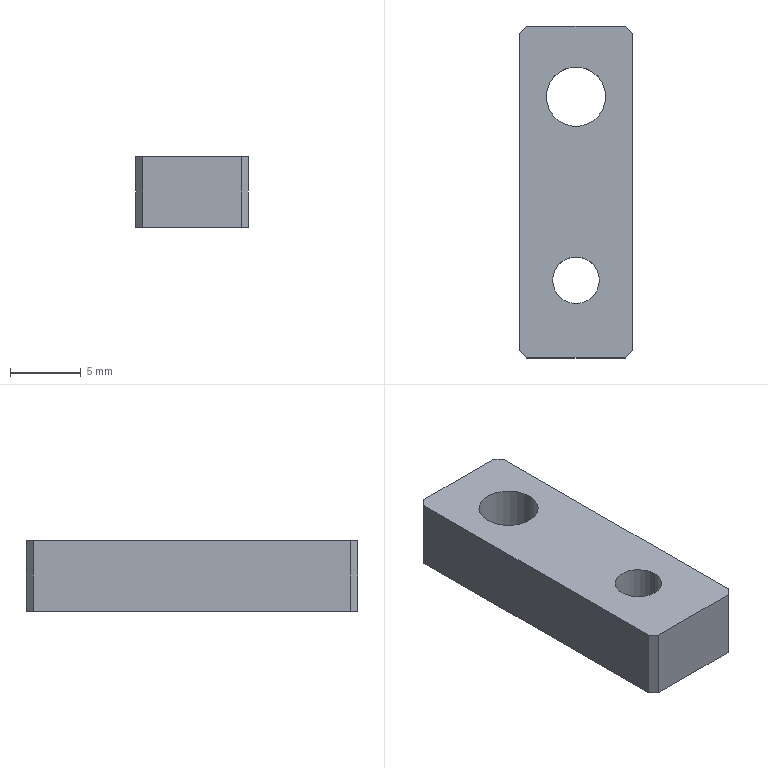Part | STEP file | 1 solid | 14 faces | box 8 x 23.5 x 5 mm | volume 825.463 mm3 | plane 10 | cylinder 4 | commonest cylinder face diameters 3.3 x2 4.2 x2
STEP:
#1=CARTESIAN_POINT('',(0.,0.,0.));
#2=DIRECTION('',(0.,0.,1.));
#3=DIRECTION('',(1.,0.,0.));
#4=AXIS2_PLACEMENT_3D('',#1,#2,#3);
#5=CARTESIAN_POINT('',(2.1,6.75,0.));
#6=VERTEX_POINT('',#5);
#7=CARTESIAN_POINT('',(2.1,6.75,5.));
#8=VERTEX_POINT('',#7);
#9=CARTESIAN_POINT('',(2.1,6.75,5.));
#10=DIRECTION('',(0.,0.,1.));
#11=VECTOR('',#10,1.);
#12=LINE('',#9,#11);
#13=CARTESIAN_POINT('',(0.,6.75,5.));
#14=DIRECTION('',(0.,0.,1.));
#15=DIRECTION('',(1.,0.,0.));
#16=AXIS2_PLACEMENT_3D('',#13,#14,#15);
#17=CYLINDRICAL_SURFACE('',#16,2.1);
#18=CARTESIAN_POINT('',(6.283,0.));
#19=DIRECTION('',(0.,1.));
#20=VECTOR('',#19,1.);
#21=LINE('',#18,#20);
#22=(GEOMETRIC_REPRESENTATION_CONTEXT(2)PARAMETRIC_REPRESENTATION_CONTEXT()REPRESENTATION_CONTEXT('',''));
#23=DEFINITIONAL_REPRESENTATION('',(#21),#22);
#24=PCURVE('',#17,#23);
#25=CARTESIAN_POINT('',(0.,6.75,5.));
#26=DIRECTION('',(0.,0.,1.));
#27=DIRECTION('',(1.,0.,0.));
#28=AXIS2_PLACEMENT_3D('',#25,#26,#27);
#29=CYLINDRICAL_SURFACE('',#28,2.1);
#30=CARTESIAN_POINT('',(0.,0.));
#31=DIRECTION('',(0.,1.));
#32=VECTOR('',#31,1.);
#33=LINE('',#30,#32);
#34=(GEOMETRIC_REPRESENTATION_CONTEXT(2)PARAMETRIC_REPRESENTATION_CONTEXT()REPRESENTATION_CONTEXT('',''));
#35=DEFINITIONAL_REPRESENTATION('',(#33),#34);
#36=PCURVE('',#29,#35);
#37=SURFACE_CURVE('',#12,(#24,#36),.PCURVE_S1.);
#38=EDGE_CURVE('',#6,#8,#37,.T.);
#39=ORIENTED_EDGE('',*,*,#38,.T.);
#40=CARTESIAN_POINT('',(-2.1,6.75,5.));
#41=VERTEX_POINT('',#40);
#42=CARTESIAN_POINT('',(0.,6.75,5.));
#43=DIRECTION('',(0.,0.,1.));
#44=DIRECTION('',(1.,0.,0.));
#45=AXIS2_PLACEMENT_3D('',#42,#43,#44);
#46=CIRCLE('',#45,2.1);
#47=CARTESIAN_POINT('',(0.,0.));
#48=DIRECTION('',(1.,0.));
#49=VECTOR('',#48,1.);
#50=LINE('',#47,#49);
#51=(GEOMETRIC_REPRESENTATION_CONTEXT(2)PARAMETRIC_REPRESENTATION_CONTEXT()REPRESENTATION_CONTEXT('',''));
#52=DEFINITIONAL_REPRESENTATION('',(#50),#51);
#53=PCURVE('',#17,#52);
#54=CARTESIAN_POINT('',(0.,0.,5.));
#55=DIRECTION('',(0.,0.,1.));
#56=DIRECTION('',(1.,0.,0.));
#57=AXIS2_PLACEMENT_3D('',#54,#55,#56);
#58=PLANE('',#57);
#59=CARTESIAN_POINT('',(0.,6.75));
#60=DIRECTION('',(1.,0.));
#61=AXIS2_PLACEMENT_2D('',#59,#60);
#62=CIRCLE('',#61,2.1);
#63=(GEOMETRIC_REPRESENTATION_CONTEXT(2)PARAMETRIC_REPRESENTATION_CONTEXT()REPRESENTATION_CONTEXT('',''));
#64=DEFINITIONAL_REPRESENTATION('',(#62),#63);
#65=PCURVE('',#58,#64);
#66=SURFACE_CURVE('',#46,(#53,#65),.PCURVE_S1.);
#67=EDGE_CURVE('',#41,#8,#66,.T.);
#68=ORIENTED_EDGE('',*,*,#67,.F.);
#69=CARTESIAN_POINT('',(-2.1,6.75,0.));
#70=VERTEX_POINT('',#69);
#71=CARTESIAN_POINT('',(-2.1,6.75,5.));
#72=DIRECTION('',(0.,0.,1.));
#73=VECTOR('',#72,1.);
#74=LINE('',#71,#73);
#75=CARTESIAN_POINT('',(3.142,0.));
#76=DIRECTION('',(0.,1.));
#77=VECTOR('',#76,1.);
#78=LINE('',#75,#77);
#79=(GEOMETRIC_REPRESENTATION_CONTEXT(2)PARAMETRIC_REPRESENTATION_CONTEXT()REPRESENTATION_CONTEXT('',''));
#80=DEFINITIONAL_REPRESENTATION('',(#78),#79);
#81=PCURVE('',#17,#80);
#82=CARTESIAN_POINT('',(3.142,0.));
#83=DIRECTION('',(0.,1.));
#84=VECTOR('',#83,1.);
#85=LINE('',#82,#84);
#86=(GEOMETRIC_REPRESENTATION_CONTEXT(2)PARAMETRIC_REPRESENTATION_CONTEXT()REPRESENTATION_CONTEXT('',''));
#87=DEFINITIONAL_REPRESENTATION('',(#85),#86);
#88=PCURVE('',#29,#87);
#89=SURFACE_CURVE('',#74,(#81,#88),.PCURVE_S1.);
#90=EDGE_CURVE('',#70,#41,#89,.T.);
#91=ORIENTED_EDGE('',*,*,#90,.F.);
#92=CARTESIAN_POINT('',(0.,6.75,0.));
#93=DIRECTION('',(0.,0.,1.));
#94=DIRECTION('',(1.,0.,0.));
#95=AXIS2_PLACEMENT_3D('',#92,#93,#94);
#96=CIRCLE('',#95,2.1);
#97=CARTESIAN_POINT('',(0.,-5.));
#98=DIRECTION('',(1.,0.));
#99=VECTOR('',#98,1.);
#100=LINE('',#97,#99);
#101=(GEOMETRIC_REPRESENTATION_CONTEXT(2)PARAMETRIC_REPRESENTATION_CONTEXT()REPRESENTATION_CONTEXT('',''));
#102=DEFINITIONAL_REPRESENTATION('',(#100),#101);
#103=PCURVE('',#17,#102);
#104=CARTESIAN_POINT('',(0.,0.,0.));
#105=DIRECTION('',(0.,0.,1.));
#106=DIRECTION('',(1.,0.,0.));
#107=AXIS2_PLACEMENT_3D('',#104,#105,#106);
#108=PLANE('',#107);
#109=CARTESIAN_POINT('',(0.,6.75));
#110=DIRECTION('',(1.,0.));
#111=AXIS2_PLACEMENT_2D('',#109,#110);
#112=CIRCLE('',#111,2.1);
#113=(GEOMETRIC_REPRESENTATION_CONTEXT(2)PARAMETRIC_REPRESENTATION_CONTEXT()REPRESENTATION_CONTEXT('',''));
#114=DEFINITIONAL_REPRESENTATION('',(#112),#113);
#115=PCURVE('',#108,#114);
#116=SURFACE_CURVE('',#96,(#103,#115),.PCURVE_S1.);
#117=EDGE_CURVE('',#70,#6,#116,.T.);
#118=ORIENTED_EDGE('',*,*,#117,.T.);
#119=EDGE_LOOP('',(#39,#68,#91,#118));
#120=FACE_BOUND('',#119,.F.);
#121=ADVANCED_FACE('',(#120),#17,.F.);
#122=CARTESIAN_POINT('',(1.65,-6.25,0.));
#123=VERTEX_POINT('',#122);
#124=CARTESIAN_POINT('',(1.65,-6.25,5.));
#125=VERTEX_POINT('',#124);
#126=CARTESIAN_POINT('',(1.65,-6.25,5.));
#127=DIRECTION('',(0.,0.,1.));
#128=VECTOR('',#127,1.);
#129=LINE('',#126,#128);
#130=CARTESIAN_POINT('',(0.,-6.25,5.));
#131=DIRECTION('',(0.,0.,1.));
#132=DIRECTION('',(1.,0.,0.));
#133=AXIS2_PLACEMENT_3D('',#130,#131,#132);
#134=CYLINDRICAL_SURFACE('',#133,1.65);
#135=CARTESIAN_POINT('',(6.283,0.));
#136=DIRECTION('',(0.,1.));
#137=VECTOR('',#136,1.);
#138=LINE('',#135,#137);
#139=(GEOMETRIC_REPRESENTATION_CONTEXT(2)PARAMETRIC_REPRESENTATION_CONTEXT()REPRESENTATION_CONTEXT('',''));
#140=DEFINITIONAL_REPRESENTATION('',(#138),#139);
#141=PCURVE('',#134,#140);
#142=CARTESIAN_POINT('',(0.,-6.25,5.));
#143=DIRECTION('',(0.,0.,1.));
#144=DIRECTION('',(1.,0.,0.));
#145=AXIS2_PLACEMENT_3D('',#142,#143,#144);
#146=CYLINDRICAL_SURFACE('',#145,1.65);
#147=CARTESIAN_POINT('',(0.,0.));
#148=DIRECTION('',(0.,1.));
#149=VECTOR('',#148,1.);
#150=LINE('',#147,#149);
#151=(GEOMETRIC_REPRESENTATION_CONTEXT(2)PARAMETRIC_REPRESENTATION_CONTEXT()REPRESENTATION_CONTEXT('',''));
#152=DEFINITIONAL_REPRESENTATION('',(#150),#151);
#153=PCURVE('',#146,#152);
#154=SURFACE_CURVE('',#129,(#141,#153),.PCURVE_S1.);
#155=EDGE_CURVE('',#123,#125,#154,.T.);
#156=ORIENTED_EDGE('',*,*,#155,.T.);
#157=CARTESIAN_POINT('',(-1.65,-6.25,5.));
#158=VERTEX_POINT('',#157);
#159=CARTESIAN_POINT('',(0.,-6.25,5.));
#160=DIRECTION('',(0.,0.,1.));
#161=DIRECTION('',(1.,0.,0.));
#162=AXIS2_PLACEMENT_3D('',#159,#160,#161);
#163=CIRCLE('',#162,1.65);
#164=CARTESIAN_POINT('',(0.,0.));
#165=DIRECTION('',(1.,0.));
#166=VECTOR('',#165,1.);
#167=LINE('',#164,#166);
#168=(GEOMETRIC_REPRESENTATION_CONTEXT(2)PARAMETRIC_REPRESENTATION_CONTEXT()REPRESENTATION_CONTEXT('',''));
#169=DEFINITIONAL_REPRESENTATION('',(#167),#168);
#170=PCURVE('',#134,#169);
#171=CARTESIAN_POINT('',(0.,-6.25));
#172=DIRECTION('',(1.,0.));
#173=AXIS2_PLACEMENT_2D('',#171,#172);
#174=CIRCLE('',#173,1.65);
#175=(GEOMETRIC_REPRESENTATION_CONTEXT(2)PARAMETRIC_REPRESENTATION_CONTEXT()REPRESENTATION_CONTEXT('',''));
#176=DEFINITIONAL_REPRESENTATION('',(#174),#175);
#177=PCURVE('',#58,#176);
#178=SURFACE_CURVE('',#163,(#170,#177),.PCURVE_S1.);
#179=EDGE_CURVE('',#158,#125,#178,.T.);
#180=ORIENTED_EDGE('',*,*,#179,.F.);
#181=CARTESIAN_POINT('',(-1.65,-6.25,0.));
#182=VERTEX_POINT('',#181);
#183=CARTESIAN_POINT('',(-1.65,-6.25,5.));
#184=DIRECTION('',(0.,0.,1.));
#185=VECTOR('',#184,1.);
#186=LINE('',#183,#185);
#187=CARTESIAN_POINT('',(3.142,0.));
#188=DIRECTION('',(0.,1.));
#189=VECTOR('',#188,1.);
#190=LINE('',#187,#189);
#191=(GEOMETRIC_REPRESENTATION_CONTEXT(2)PARAMETRIC_REPRESENTATION_CONTEXT()REPRESENTATION_CONTEXT('',''));
#192=DEFINITIONAL_REPRESENTATION('',(#190),#191);
#193=PCURVE('',#134,#192);
#194=CARTESIAN_POINT('',(3.142,0.));
#195=DIRECTION('',(0.,1.));
#196=VECTOR('',#195,1.);
#197=LINE('',#194,#196);
#198=(GEOMETRIC_REPRESENTATION_CONTEXT(2)PARAMETRIC_REPRESENTATION_CONTEXT()REPRESENTATION_CONTEXT('',''));
#199=DEFINITIONAL_REPRESENTATION('',(#197),#198);
#200=PCURVE('',#146,#199);
#201=SURFACE_CURVE('',#186,(#193,#200),.PCURVE_S1.);
#202=EDGE_CURVE('',#182,#158,#201,.T.);
#203=ORIENTED_EDGE('',*,*,#202,.F.);
#204=CARTESIAN_POINT('',(0.,-6.25,0.));
#205=DIRECTION('',(0.,0.,1.));
#206=DIRECTION('',(1.,0.,0.));
#207=AXIS2_PLACEMENT_3D('',#204,#205,#206);
#208=CIRCLE('',#207,1.65);
#209=CARTESIAN_POINT('',(0.,-5.));
#210=DIRECTION('',(1.,0.));
#211=VECTOR('',#210,1.);
#212=LINE('',#209,#211);
#213=(GEOMETRIC_REPRESENTATION_CONTEXT(2)PARAMETRIC_REPRESENTATION_CONTEXT()REPRESENTATION_CONTEXT('',''));
#214=DEFINITIONAL_REPRESENTATION('',(#212),#213);
#215=PCURVE('',#134,#214);
#216=CARTESIAN_POINT('',(0.,-6.25));
#217=DIRECTION('',(1.,0.));
#218=AXIS2_PLACEMENT_2D('',#216,#217);
#219=CIRCLE('',#218,1.65);
#220=(GEOMETRIC_REPRESENTATION_CONTEXT(2)PARAMETRIC_REPRESENTATION_CONTEXT()REPRESENTATION_CONTEXT('',''));
#221=DEFINITIONAL_REPRESENTATION('',(#219),#220);
#222=PCURVE('',#108,#221);
#223=SURFACE_CURVE('',#208,(#215,#222),.PCURVE_S1.);
#224=EDGE_CURVE('',#182,#123,#223,.T.);
#225=ORIENTED_EDGE('',*,*,#224,.T.);
#226=EDGE_LOOP('',(#156,#180,#203,#225));
#227=FACE_BOUND('',#226,.F.);
#228=ADVANCED_FACE('',(#227),#134,.F.);
#229=CARTESIAN_POINT('',(4.,-11.25,5.));
#230=VERTEX_POINT('',#229);
#231=CARTESIAN_POINT('',(4.,11.25,5.));
#232=VERTEX_POINT('',#231);
#233=CARTESIAN_POINT('',(4.,11.75,5.));
#234=DIRECTION('',(0.,1.,0.));
#235=VECTOR('',#234,1.);
#236=LINE('',#233,#235);
#237=CARTESIAN_POINT('',(4.,11.75,5.));
#238=DIRECTION('',(-1.,0.,0.));
#239=DIRECTION('',(0.,-1.,0.));
#240=AXIS2_PLACEMENT_3D('',#237,#238,#239);
#241=PLANE('',#240);
#242=CARTESIAN_POINT('',(0.,0.));
#243=DIRECTION('',(-1.,0.));
#244=VECTOR('',#243,1.);
#245=LINE('',#242,#244);
#246=(GEOMETRIC_REPRESENTATION_CONTEXT(2)PARAMETRIC_REPRESENTATION_CONTEXT()REPRESENTATION_CONTEXT('',''));
#247=DEFINITIONAL_REPRESENTATION('',(#245),#246);
#248=PCURVE('',#241,#247);
#249=CARTESIAN_POINT('',(4.,11.75));
#250=DIRECTION('',(0.,1.));
#251=VECTOR('',#250,1.);
#252=LINE('',#249,#251);
#253=(GEOMETRIC_REPRESENTATION_CONTEXT(2)PARAMETRIC_REPRESENTATION_CONTEXT()REPRESENTATION_CONTEXT('',''));
#254=DEFINITIONAL_REPRESENTATION('',(#252),#253);
#255=PCURVE('',#58,#254);
#256=SURFACE_CURVE('',#236,(#248,#255),.PCURVE_S1.);
#257=EDGE_CURVE('',#230,#232,#256,.T.);
#258=ORIENTED_EDGE('',*,*,#257,.F.);
#259=CARTESIAN_POINT('',(4.,-11.25,0.));
#260=VERTEX_POINT('',#259);
#261=CARTESIAN_POINT('',(4.,-11.25,5.));
#262=DIRECTION('',(0.,0.,-1.));
#263=VECTOR('',#262,1.);
#264=LINE('',#261,#263);
#265=CARTESIAN_POINT('',(23.,0.));
#266=DIRECTION('',(0.,-1.));
#267=VECTOR('',#266,1.);
#268=LINE('',#265,#267);
#269=(GEOMETRIC_REPRESENTATION_CONTEXT(2)PARAMETRIC_REPRESENTATION_CONTEXT()REPRESENTATION_CONTEXT('',''));
#270=DEFINITIONAL_REPRESENTATION('',(#268),#269);
#271=PCURVE('',#241,#270);
#272=CARTESIAN_POINT('',(4.,-11.25,5.));
#273=DIRECTION('',(-0.7071,0.7071,0.));
#274=DIRECTION('',(0.,0.,-1.));
#275=AXIS2_PLACEMENT_3D('',#272,#273,#274);
#276=PLANE('',#275);
#277=CARTESIAN_POINT('',(0.,0.));
#278=DIRECTION('',(1.,0.));
#279=VECTOR('',#278,1.);
#280=LINE('',#277,#279);
#281=(GEOMETRIC_REPRESENTATION_CONTEXT(2)PARAMETRIC_REPRESENTATION_CONTEXT()REPRESENTATION_CONTEXT('',''));
#282=DEFINITIONAL_REPRESENTATION('',(#280),#281);
#283=PCURVE('',#276,#282);
#284=SURFACE_CURVE('',#264,(#271,#283),.PCURVE_S1.);
#285=EDGE_CURVE('',#230,#260,#284,.T.);
#286=ORIENTED_EDGE('',*,*,#285,.T.);
#287=CARTESIAN_POINT('',(4.,11.25,0.));
#288=VERTEX_POINT('',#287);
#289=CARTESIAN_POINT('',(4.,11.75,0.));
#290=DIRECTION('',(0.,1.,0.));
#291=VECTOR('',#290,1.);
#292=LINE('',#289,#291);
#293=CARTESIAN_POINT('',(0.,-5.));
#294=DIRECTION('',(-1.,0.));
#295=VECTOR('',#294,1.);
#296=LINE('',#293,#295);
#297=(GEOMETRIC_REPRESENTATION_CONTEXT(2)PARAMETRIC_REPRESENTATION_CONTEXT()REPRESENTATION_CONTEXT('',''));
#298=DEFINITIONAL_REPRESENTATION('',(#296),#297);
#299=PCURVE('',#241,#298);
#300=CARTESIAN_POINT('',(4.,11.75));
#301=DIRECTION('',(0.,1.));
#302=VECTOR('',#301,1.);
#303=LINE('',#300,#302);
#304=(GEOMETRIC_REPRESENTATION_CONTEXT(2)PARAMETRIC_REPRESENTATION_CONTEXT()REPRESENTATION_CONTEXT('',''));
#305=DEFINITIONAL_REPRESENTATION('',(#303),#304);
#306=PCURVE('',#108,#305);
#307=SURFACE_CURVE('',#292,(#299,#306),.PCURVE_S1.);
#308=EDGE_CURVE('',#260,#288,#307,.T.);
#309=ORIENTED_EDGE('',*,*,#308,.T.);
#310=CARTESIAN_POINT('',(4.,11.25,5.));
#311=DIRECTION('',(0.,0.,1.));
#312=VECTOR('',#311,1.);
#313=LINE('',#310,#312);
#314=CARTESIAN_POINT('',(0.5,0.));
#315=DIRECTION('',(0.,1.));
#316=VECTOR('',#315,1.);
#317=LINE('',#314,#316);
#318=(GEOMETRIC_REPRESENTATION_CONTEXT(2)PARAMETRIC_REPRESENTATION_CONTEXT()REPRESENTATION_CONTEXT('',''));
#319=DEFINITIONAL_REPRESENTATION('',(#317),#318);
#320=PCURVE('',#241,#319);
#321=CARTESIAN_POINT('',(3.5,11.75,5.));
#322=DIRECTION('',(-0.7071,-0.7071,0.));
#323=DIRECTION('',(0.,0.,-1.));
#324=AXIS2_PLACEMENT_3D('',#321,#322,#323);
#325=PLANE('',#324);
#326=CARTESIAN_POINT('',(0.,0.7071));
#327=DIRECTION('',(-1.,0.));
#328=VECTOR('',#327,1.);
#329=LINE('',#326,#328);
#330=(GEOMETRIC_REPRESENTATION_CONTEXT(2)PARAMETRIC_REPRESENTATION_CONTEXT()REPRESENTATION_CONTEXT('',''));
#331=DEFINITIONAL_REPRESENTATION('',(#329),#330);
#332=PCURVE('',#325,#331);
#333=SURFACE_CURVE('',#313,(#320,#332),.PCURVE_S1.);
#334=EDGE_CURVE('',#288,#232,#333,.T.);
#335=ORIENTED_EDGE('',*,*,#334,.T.);
#336=EDGE_LOOP('',(#258,#286,#309,#335));
#337=FACE_BOUND('',#336,.T.);
#338=ADVANCED_FACE('',(#337),#241,.F.);
#339=CARTESIAN_POINT('',(3.5,11.75,0.));
#340=VERTEX_POINT('',#339);
#341=CARTESIAN_POINT('',(-3.5,11.75,0.));
#342=VERTEX_POINT('',#341);
#343=CARTESIAN_POINT('',(-4.,11.75,0.));
#344=DIRECTION('',(-1.,0.,0.));
#345=VECTOR('',#344,1.);
#346=LINE('',#343,#345);
#347=CARTESIAN_POINT('',(-4.,11.75,5.));
#348=DIRECTION('',(0.,-1.,0.));
#349=DIRECTION('',(0.,0.,-1.));
#350=AXIS2_PLACEMENT_3D('',#347,#348,#349);
#351=PLANE('',#350);
#352=CARTESIAN_POINT('',(5.,0.));
#353=DIRECTION('',(0.,-1.));
#354=VECTOR('',#353,1.);
#355=LINE('',#352,#354);
#356=(GEOMETRIC_REPRESENTATION_CONTEXT(2)PARAMETRIC_REPRESENTATION_CONTEXT()REPRESENTATION_CONTEXT('',''));
#357=DEFINITIONAL_REPRESENTATION('',(#355),#356);
#358=PCURVE('',#351,#357);
#359=CARTESIAN_POINT('',(-4.,11.75));
#360=DIRECTION('',(-1.,0.));
#361=VECTOR('',#360,1.);
#362=LINE('',#359,#361);
#363=(GEOMETRIC_REPRESENTATION_CONTEXT(2)PARAMETRIC_REPRESENTATION_CONTEXT()REPRESENTATION_CONTEXT('',''));
#364=DEFINITIONAL_REPRESENTATION('',(#362),#363);
#365=PCURVE('',#108,#364);
#366=SURFACE_CURVE('',#346,(#358,#365),.PCURVE_S1.);
#367=EDGE_CURVE('',#340,#342,#366,.T.);
#368=ORIENTED_EDGE('',*,*,#367,.T.);
#369=CARTESIAN_POINT('',(-3.5,11.75,5.));
#370=VERTEX_POINT('',#369);
#371=CARTESIAN_POINT('',(-3.5,11.75,5.));
#372=DIRECTION('',(0.,0.,1.));
#373=VECTOR('',#372,1.);
#374=LINE('',#371,#373);
#375=CARTESIAN_POINT('',(0.,0.5));
#376=DIRECTION('',(-1.,0.));
#377=VECTOR('',#376,1.);
#378=LINE('',#375,#377);
#379=(GEOMETRIC_REPRESENTATION_CONTEXT(2)PARAMETRIC_REPRESENTATION_CONTEXT()REPRESENTATION_CONTEXT('',''));
#380=DEFINITIONAL_REPRESENTATION('',(#378),#379);
#381=PCURVE('',#351,#380);
#382=CARTESIAN_POINT('',(-4.,11.25,5.));
#383=DIRECTION('',(0.7071,-0.7071,0.));
#384=DIRECTION('',(0.,0.,-1.));
#385=AXIS2_PLACEMENT_3D('',#382,#383,#384);
#386=PLANE('',#385);
#387=CARTESIAN_POINT('',(0.,0.7071));
#388=DIRECTION('',(-1.,0.));
#389=VECTOR('',#388,1.);
#390=LINE('',#387,#389);
#391=(GEOMETRIC_REPRESENTATION_CONTEXT(2)PARAMETRIC_REPRESENTATION_CONTEXT()REPRESENTATION_CONTEXT('',''));
#392=DEFINITIONAL_REPRESENTATION('',(#390),#391);
#393=PCURVE('',#386,#392);
#394=SURFACE_CURVE('',#374,(#381,#393),.PCURVE_S1.);
#395=EDGE_CURVE('',#342,#370,#394,.T.);
#396=ORIENTED_EDGE('',*,*,#395,.T.);
#397=CARTESIAN_POINT('',(3.5,11.75,5.));
#398=VERTEX_POINT('',#397);
#399=CARTESIAN_POINT('',(-4.,11.75,5.));
#400=DIRECTION('',(-1.,0.,0.));
#401=VECTOR('',#400,1.);
#402=LINE('',#399,#401);
#403=CARTESIAN_POINT('',(0.,0.));
#404=DIRECTION('',(0.,-1.));
#405=VECTOR('',#404,1.);
#406=LINE('',#403,#405);
#407=(GEOMETRIC_REPRESENTATION_CONTEXT(2)PARAMETRIC_REPRESENTATION_CONTEXT()REPRESENTATION_CONTEXT('',''));
#408=DEFINITIONAL_REPRESENTATION('',(#406),#407);
#409=PCURVE('',#351,#408);
#410=CARTESIAN_POINT('',(-4.,11.75));
#411=DIRECTION('',(-1.,0.));
#412=VECTOR('',#411,1.);
#413=LINE('',#410,#412);
#414=(GEOMETRIC_REPRESENTATION_CONTEXT(2)PARAMETRIC_REPRESENTATION_CONTEXT()REPRESENTATION_CONTEXT('',''));
#415=DEFINITIONAL_REPRESENTATION('',(#413),#414);
#416=PCURVE('',#58,#415);
#417=SURFACE_CURVE('',#402,(#409,#416),.PCURVE_S1.);
#418=EDGE_CURVE('',#398,#370,#417,.T.);
#419=ORIENTED_EDGE('',*,*,#418,.F.);
#420=CARTESIAN_POINT('',(3.5,11.75,5.));
#421=DIRECTION('',(0.,0.,-1.));
#422=VECTOR('',#421,1.);
#423=LINE('',#420,#422);
#424=CARTESIAN_POINT('',(0.,7.5));
#425=DIRECTION('',(1.,0.));
#426=VECTOR('',#425,1.);
#427=LINE('',#424,#426);
#428=(GEOMETRIC_REPRESENTATION_CONTEXT(2)PARAMETRIC_REPRESENTATION_CONTEXT()REPRESENTATION_CONTEXT('',''));
#429=DEFINITIONAL_REPRESENTATION('',(#427),#428);
#430=PCURVE('',#351,#429);
#431=CARTESIAN_POINT('',(0.,0.));
#432=DIRECTION('',(1.,0.));
#433=VECTOR('',#432,1.);
#434=LINE('',#431,#433);
#435=(GEOMETRIC_REPRESENTATION_CONTEXT(2)PARAMETRIC_REPRESENTATION_CONTEXT()REPRESENTATION_CONTEXT('',''));
#436=DEFINITIONAL_REPRESENTATION('',(#434),#435);
#437=PCURVE('',#325,#436);
#438=SURFACE_CURVE('',#423,(#430,#437),.PCURVE_S1.);
#439=EDGE_CURVE('',#398,#340,#438,.T.);
#440=ORIENTED_EDGE('',*,*,#439,.T.);
#441=EDGE_LOOP('',(#368,#396,#419,#440));
#442=FACE_BOUND('',#441,.T.);
#443=ADVANCED_FACE('',(#442),#351,.F.);
#444=CARTESIAN_POINT('',(-4.,11.25,0.));
#445=VERTEX_POINT('',#444);
#446=CARTESIAN_POINT('',(-4.,-11.25,0.));
#447=VERTEX_POINT('',#446);
#448=CARTESIAN_POINT('',(-4.,11.75,0.));
#449=DIRECTION('',(0.,-1.,0.));
#450=VECTOR('',#449,1.);
#451=LINE('',#448,#450);
#452=CARTESIAN_POINT('',(-4.,11.75,5.));
#453=DIRECTION('',(1.,0.,0.));
#454=DIRECTION('',(0.,1.,0.));
#455=AXIS2_PLACEMENT_3D('',#452,#453,#454);
#456=PLANE('',#455);
#457=CARTESIAN_POINT('',(0.,-5.));
#458=DIRECTION('',(-1.,0.));
#459=VECTOR('',#458,1.);
#460=LINE('',#457,#459);
#461=(GEOMETRIC_REPRESENTATION_CONTEXT(2)PARAMETRIC_REPRESENTATION_CONTEXT()REPRESENTATION_CONTEXT('',''));
#462=DEFINITIONAL_REPRESENTATION('',(#460),#461);
#463=PCURVE('',#456,#462);
#464=CARTESIAN_POINT('',(-4.,11.75));
#465=DIRECTION('',(0.,-1.));
#466=VECTOR('',#465,1.);
#467=LINE('',#464,#466);
#468=(GEOMETRIC_REPRESENTATION_CONTEXT(2)PARAMETRIC_REPRESENTATION_CONTEXT()REPRESENTATION_CONTEXT('',''));
#469=DEFINITIONAL_REPRESENTATION('',(#467),#468);
#470=PCURVE('',#108,#469);
#471=SURFACE_CURVE('',#451,(#463,#470),.PCURVE_S1.);
#472=EDGE_CURVE('',#445,#447,#471,.T.);
#473=ORIENTED_EDGE('',*,*,#472,.T.);
#474=CARTESIAN_POINT('',(-4.,-11.25,5.));
#475=VERTEX_POINT('',#474);
#476=CARTESIAN_POINT('',(-4.,-11.25,5.));
#477=DIRECTION('',(0.,0.,1.));
#478=VECTOR('',#477,1.);
#479=LINE('',#476,#478);
#480=CARTESIAN_POINT('',(-23.,0.));
#481=DIRECTION('',(0.,1.));
#482=VECTOR('',#481,1.);
#483=LINE('',#480,#482);
#484=(GEOMETRIC_REPRESENTATION_CONTEXT(2)PARAMETRIC_REPRESENTATION_CONTEXT()REPRESENTATION_CONTEXT('',''));
#485=DEFINITIONAL_REPRESENTATION('',(#483),#484);
#486=PCURVE('',#456,#485);
#487=CARTESIAN_POINT('',(-3.5,-11.75,5.));
#488=DIRECTION('',(0.7071,0.7071,0.));
#489=DIRECTION('',(0.,0.,-1.));
#490=AXIS2_PLACEMENT_3D('',#487,#488,#489);
#491=PLANE('',#490);
#492=CARTESIAN_POINT('',(0.,0.7071));
#493=DIRECTION('',(-1.,0.));
#494=VECTOR('',#493,1.);
#495=LINE('',#492,#494);
#496=(GEOMETRIC_REPRESENTATION_CONTEXT(2)PARAMETRIC_REPRESENTATION_CONTEXT()REPRESENTATION_CONTEXT('',''));
#497=DEFINITIONAL_REPRESENTATION('',(#495),#496);
#498=PCURVE('',#491,#497);
#499=SURFACE_CURVE('',#479,(#486,#498),.PCURVE_S1.);
#500=EDGE_CURVE('',#447,#475,#499,.T.);
#501=ORIENTED_EDGE('',*,*,#500,.T.);
#502=CARTESIAN_POINT('',(-4.,11.25,5.));
#503=VERTEX_POINT('',#502);
#504=CARTESIAN_POINT('',(-4.,11.75,5.));
#505=DIRECTION('',(0.,-1.,0.));
#506=VECTOR('',#505,1.);
#507=LINE('',#504,#506);
#508=CARTESIAN_POINT('',(0.,0.));
#509=DIRECTION('',(-1.,0.));
#510=VECTOR('',#509,1.);
#511=LINE('',#508,#510);
#512=(GEOMETRIC_REPRESENTATION_CONTEXT(2)PARAMETRIC_REPRESENTATION_CONTEXT()REPRESENTATION_CONTEXT('',''));
#513=DEFINITIONAL_REPRESENTATION('',(#511),#512);
#514=PCURVE('',#456,#513);
#515=CARTESIAN_POINT('',(-4.,11.75));
#516=DIRECTION('',(0.,-1.));
#517=VECTOR('',#516,1.);
#518=LINE('',#515,#517);
#519=(GEOMETRIC_REPRESENTATION_CONTEXT(2)PARAMETRIC_REPRESENTATION_CONTEXT()REPRESENTATION_CONTEXT('',''));
#520=DEFINITIONAL_REPRESENTATION('',(#518),#519);
#521=PCURVE('',#58,#520);
#522=SURFACE_CURVE('',#507,(#514,#521),.PCURVE_S1.);
#523=EDGE_CURVE('',#503,#475,#522,.T.);
#524=ORIENTED_EDGE('',*,*,#523,.F.);
#525=CARTESIAN_POINT('',(-4.,11.25,5.));
#526=DIRECTION('',(0.,0.,-1.));
#527=VECTOR('',#526,1.);
#528=LINE('',#525,#527);
#529=CARTESIAN_POINT('',(-0.5,0.));
#530=DIRECTION('',(0.,-1.));
#531=VECTOR('',#530,1.);
#532=LINE('',#529,#531);
#533=(GEOMETRIC_REPRESENTATION_CONTEXT(2)PARAMETRIC_REPRESENTATION_CONTEXT()REPRESENTATION_CONTEXT('',''));
#534=DEFINITIONAL_REPRESENTATION('',(#532),#533);
#535=PCURVE('',#456,#534);
#536=CARTESIAN_POINT('',(0.,0.));
#537=DIRECTION('',(1.,0.));
#538=VECTOR('',#537,1.);
#539=LINE('',#536,#538);
#540=(GEOMETRIC_REPRESENTATION_CONTEXT(2)PARAMETRIC_REPRESENTATION_CONTEXT()REPRESENTATION_CONTEXT('',''));
#541=DEFINITIONAL_REPRESENTATION('',(#539),#540);
#542=PCURVE('',#386,#541);
#543=SURFACE_CURVE('',#528,(#535,#542),.PCURVE_S1.);
#544=EDGE_CURVE('',#503,#445,#543,.T.);
#545=ORIENTED_EDGE('',*,*,#544,.T.);
#546=EDGE_LOOP('',(#473,#501,#524,#545));
#547=FACE_BOUND('',#546,.T.);
#548=ADVANCED_FACE('',(#547),#456,.F.);
#549=CARTESIAN_POINT('',(-3.5,-11.75,5.));
#550=VERTEX_POINT('',#549);
#551=CARTESIAN_POINT('',(3.5,-11.75,5.));
#552=VERTEX_POINT('',#551);
#553=CARTESIAN_POINT('',(-4.,-11.75,5.));
#554=DIRECTION('',(1.,0.,0.));
#555=VECTOR('',#554,1.);
#556=LINE('',#553,#555);
#557=CARTESIAN_POINT('',(-4.,-11.75,5.));
#558=DIRECTION('',(0.,1.,0.));
#559=DIRECTION('',(0.,0.,1.));
#560=AXIS2_PLACEMENT_3D('',#557,#558,#559);
#561=PLANE('',#560);
#562=CARTESIAN_POINT('',(0.,0.));
#563=DIRECTION('',(0.,1.));
#564=VECTOR('',#563,1.);
#565=LINE('',#562,#564);
#566=(GEOMETRIC_REPRESENTATION_CONTEXT(2)PARAMETRIC_REPRESENTATION_CONTEXT()REPRESENTATION_CONTEXT('',''));
#567=DEFINITIONAL_REPRESENTATION('',(#565),#566);
#568=PCURVE('',#561,#567);
#569=CARTESIAN_POINT('',(-4.,-11.75));
#570=DIRECTION('',(1.,0.));
#571=VECTOR('',#570,1.);
#572=LINE('',#569,#571);
#573=(GEOMETRIC_REPRESENTATION_CONTEXT(2)PARAMETRIC_REPRESENTATION_CONTEXT()REPRESENTATION_CONTEXT('',''));
#574=DEFINITIONAL_REPRESENTATION('',(#572),#573);
#575=PCURVE('',#58,#574);
#576=SURFACE_CURVE('',#556,(#568,#575),.PCURVE_S1.);
#577=EDGE_CURVE('',#550,#552,#576,.T.);
#578=ORIENTED_EDGE('',*,*,#577,.F.);
#579=CARTESIAN_POINT('',(-3.5,-11.75,0.));
#580=VERTEX_POINT('',#579);
#581=CARTESIAN_POINT('',(-3.5,-11.75,5.));
#582=DIRECTION('',(0.,0.,-1.));
#583=VECTOR('',#582,1.);
#584=LINE('',#581,#583);
#585=CARTESIAN_POINT('',(0.,0.5));
#586=DIRECTION('',(-1.,0.));
#587=VECTOR('',#586,1.);
#588=LINE('',#585,#587);
#589=(GEOMETRIC_REPRESENTATION_CONTEXT(2)PARAMETRIC_REPRESENTATION_CONTEXT()REPRESENTATION_CONTEXT('',''));
#590=DEFINITIONAL_REPRESENTATION('',(#588),#589);
#591=PCURVE('',#561,#590);
#592=CARTESIAN_POINT('',(0.,0.));
#593=DIRECTION('',(1.,0.));
#594=VECTOR('',#593,1.);
#595=LINE('',#592,#594);
#596=(GEOMETRIC_REPRESENTATION_CONTEXT(2)PARAMETRIC_REPRESENTATION_CONTEXT()REPRESENTATION_CONTEXT('',''));
#597=DEFINITIONAL_REPRESENTATION('',(#595),#596);
#598=PCURVE('',#491,#597);
#599=SURFACE_CURVE('',#584,(#591,#598),.PCURVE_S1.);
#600=EDGE_CURVE('',#550,#580,#599,.T.);
#601=ORIENTED_EDGE('',*,*,#600,.T.);
#602=CARTESIAN_POINT('',(3.5,-11.75,0.));
#603=VERTEX_POINT('',#602);
#604=CARTESIAN_POINT('',(-4.,-11.75,0.));
#605=DIRECTION('',(1.,0.,0.));
#606=VECTOR('',#605,1.);
#607=LINE('',#604,#606);
#608=CARTESIAN_POINT('',(-5.,0.));
#609=DIRECTION('',(0.,1.));
#610=VECTOR('',#609,1.);
#611=LINE('',#608,#610);
#612=(GEOMETRIC_REPRESENTATION_CONTEXT(2)PARAMETRIC_REPRESENTATION_CONTEXT()REPRESENTATION_CONTEXT('',''));
#613=DEFINITIONAL_REPRESENTATION('',(#611),#612);
#614=PCURVE('',#561,#613);
#615=CARTESIAN_POINT('',(-4.,-11.75));
#616=DIRECTION('',(1.,0.));
#617=VECTOR('',#616,1.);
#618=LINE('',#615,#617);
#619=(GEOMETRIC_REPRESENTATION_CONTEXT(2)PARAMETRIC_REPRESENTATION_CONTEXT()REPRESENTATION_CONTEXT('',''));
#620=DEFINITIONAL_REPRESENTATION('',(#618),#619);
#621=PCURVE('',#108,#620);
#622=SURFACE_CURVE('',#607,(#614,#621),.PCURVE_S1.);
#623=EDGE_CURVE('',#580,#603,#622,.T.);
#624=ORIENTED_EDGE('',*,*,#623,.T.);
#625=CARTESIAN_POINT('',(3.5,-11.75,5.));
#626=DIRECTION('',(0.,0.,1.));
#627=VECTOR('',#626,1.);
#628=LINE('',#625,#627);
#629=CARTESIAN_POINT('',(0.,7.5));
#630=DIRECTION('',(1.,0.));
#631=VECTOR('',#630,1.);
#632=LINE('',#629,#631);
#633=(GEOMETRIC_REPRESENTATION_CONTEXT(2)PARAMETRIC_REPRESENTATION_CONTEXT()REPRESENTATION_CONTEXT('',''));
#634=DEFINITIONAL_REPRESENTATION('',(#632),#633);
#635=PCURVE('',#561,#634);
#636=CARTESIAN_POINT('',(0.,0.7071));
#637=DIRECTION('',(-1.,0.));
#638=VECTOR('',#637,1.);
#639=LINE('',#636,#638);
#640=(GEOMETRIC_REPRESENTATION_CONTEXT(2)PARAMETRIC_REPRESENTATION_CONTEXT()REPRESENTATION_CONTEXT('',''));
#641=DEFINITIONAL_REPRESENTATION('',(#639),#640);
#642=PCURVE('',#276,#641);
#643=SURFACE_CURVE('',#628,(#635,#642),.PCURVE_S1.);
#644=EDGE_CURVE('',#603,#552,#643,.T.);
#645=ORIENTED_EDGE('',*,*,#644,.T.);
#646=EDGE_LOOP('',(#578,#601,#624,#645));
#647=FACE_BOUND('',#646,.T.);
#648=ADVANCED_FACE('',(#647),#561,.F.);
#649=CARTESIAN_POINT('',(0.,6.75,5.));
#650=DIRECTION('',(0.,0.,1.));
#651=DIRECTION('',(1.,0.,0.));
#652=AXIS2_PLACEMENT_3D('',#649,#650,#651);
#653=CIRCLE('',#652,2.1);
#654=CARTESIAN_POINT('',(0.,6.75));
#655=DIRECTION('',(1.,0.));
#656=AXIS2_PLACEMENT_2D('',#654,#655);
#657=CIRCLE('',#656,2.1);
#658=(GEOMETRIC_REPRESENTATION_CONTEXT(2)PARAMETRIC_REPRESENTATION_CONTEXT()REPRESENTATION_CONTEXT('',''));
#659=DEFINITIONAL_REPRESENTATION('',(#657),#658);
#660=PCURVE('',#58,#659);
#661=CARTESIAN_POINT('',(0.,0.));
#662=DIRECTION('',(1.,0.));
#663=VECTOR('',#662,1.);
#664=LINE('',#661,#663);
#665=(GEOMETRIC_REPRESENTATION_CONTEXT(2)PARAMETRIC_REPRESENTATION_CONTEXT()REPRESENTATION_CONTEXT('',''));
#666=DEFINITIONAL_REPRESENTATION('',(#664),#665);
#667=PCURVE('',#29,#666);
#668=SURFACE_CURVE('',#653,(#660,#667),.PCURVE_S1.);
#669=EDGE_CURVE('',#8,#41,#668,.T.);
#670=ORIENTED_EDGE('',*,*,#669,.F.);
#671=ORIENTED_EDGE('',*,*,#67,.F.);
#672=EDGE_LOOP('',(#670,#671));
#673=FACE_BOUND('',#672,.T.);
#674=CARTESIAN_POINT('',(0.,-6.25,5.));
#675=DIRECTION('',(0.,0.,1.));
#676=DIRECTION('',(1.,0.,0.));
#677=AXIS2_PLACEMENT_3D('',#674,#675,#676);
#678=CIRCLE('',#677,1.65);
#679=CARTESIAN_POINT('',(0.,-6.25));
#680=DIRECTION('',(1.,0.));
#681=AXIS2_PLACEMENT_2D('',#679,#680);
#682=CIRCLE('',#681,1.65);
#683=(GEOMETRIC_REPRESENTATION_CONTEXT(2)PARAMETRIC_REPRESENTATION_CONTEXT()REPRESENTATION_CONTEXT('',''));
#684=DEFINITIONAL_REPRESENTATION('',(#682),#683);
#685=PCURVE('',#58,#684);
#686=CARTESIAN_POINT('',(0.,0.));
#687=DIRECTION('',(1.,0.));
#688=VECTOR('',#687,1.);
#689=LINE('',#686,#688);
#690=(GEOMETRIC_REPRESENTATION_CONTEXT(2)PARAMETRIC_REPRESENTATION_CONTEXT()REPRESENTATION_CONTEXT('',''));
#691=DEFINITIONAL_REPRESENTATION('',(#689),#690);
#692=PCURVE('',#146,#691);
#693=SURFACE_CURVE('',#678,(#685,#692),.PCURVE_S1.);
#694=EDGE_CURVE('',#125,#158,#693,.T.);
#695=ORIENTED_EDGE('',*,*,#694,.F.);
#696=ORIENTED_EDGE('',*,*,#179,.F.);
#697=EDGE_LOOP('',(#695,#696));
#698=FACE_BOUND('',#697,.T.);
#699=ORIENTED_EDGE('',*,*,#523,.T.);
#700=CARTESIAN_POINT('',(-7.625,-7.625,5.));
#701=DIRECTION('',(0.7071,-0.7071,0.));
#702=VECTOR('',#701,1.);
#703=LINE('',#700,#702);
#704=CARTESIAN_POINT('',(-7.625,-7.625));
#705=DIRECTION('',(0.7071,-0.7071));
#706=VECTOR('',#705,1.);
#707=LINE('',#704,#706);
#708=(GEOMETRIC_REPRESENTATION_CONTEXT(2)PARAMETRIC_REPRESENTATION_CONTEXT()REPRESENTATION_CONTEXT('',''));
#709=DEFINITIONAL_REPRESENTATION('',(#707),#708);
#710=PCURVE('',#58,#709);
#711=CARTESIAN_POINT('',(0.,5.834));
#712=DIRECTION('',(0.,-1.));
#713=VECTOR('',#712,1.);
#714=LINE('',#711,#713);
#715=(GEOMETRIC_REPRESENTATION_CONTEXT(2)PARAMETRIC_REPRESENTATION_CONTEXT()REPRESENTATION_CONTEXT('',''));
#716=DEFINITIONAL_REPRESENTATION('',(#714),#715);
#717=PCURVE('',#491,#716);
#718=SURFACE_CURVE('',#703,(#710,#717),.PCURVE_S1.);
#719=EDGE_CURVE('',#475,#550,#718,.T.);
#720=ORIENTED_EDGE('',*,*,#719,.T.);
#721=ORIENTED_EDGE('',*,*,#577,.T.);
#722=CARTESIAN_POINT('',(7.625,-7.625,5.));
#723=DIRECTION('',(0.7071,0.7071,0.));
#724=VECTOR('',#723,1.);
#725=LINE('',#722,#724);
#726=CARTESIAN_POINT('',(7.625,-7.625));
#727=DIRECTION('',(0.7071,0.7071));
#728=VECTOR('',#727,1.);
#729=LINE('',#726,#728);
#730=(GEOMETRIC_REPRESENTATION_CONTEXT(2)PARAMETRIC_REPRESENTATION_CONTEXT()REPRESENTATION_CONTEXT('',''));
#731=DEFINITIONAL_REPRESENTATION('',(#729),#730);
#732=PCURVE('',#58,#731);
#733=CARTESIAN_POINT('',(0.,-5.127));
#734=DIRECTION('',(0.,-1.));
#735=VECTOR('',#734,1.);
#736=LINE('',#733,#735);
#737=(GEOMETRIC_REPRESENTATION_CONTEXT(2)PARAMETRIC_REPRESENTATION_CONTEXT()REPRESENTATION_CONTEXT('',''));
#738=DEFINITIONAL_REPRESENTATION('',(#736),#737);
#739=PCURVE('',#276,#738);
#740=SURFACE_CURVE('',#725,(#732,#739),.PCURVE_S1.);
#741=EDGE_CURVE('',#552,#230,#740,.T.);
#742=ORIENTED_EDGE('',*,*,#741,.T.);
#743=ORIENTED_EDGE('',*,*,#257,.T.);
#744=CARTESIAN_POINT('',(7.625,7.625,5.));
#745=DIRECTION('',(-0.7071,0.7071,0.));
#746=VECTOR('',#745,1.);
#747=LINE('',#744,#746);
#748=CARTESIAN_POINT('',(7.625,7.625));
#749=DIRECTION('',(-0.7071,0.7071));
#750=VECTOR('',#749,1.);
#751=LINE('',#748,#750);
#752=(GEOMETRIC_REPRESENTATION_CONTEXT(2)PARAMETRIC_REPRESENTATION_CONTEXT()REPRESENTATION_CONTEXT('',''));
#753=DEFINITIONAL_REPRESENTATION('',(#751),#752);
#754=PCURVE('',#58,#753);
#755=CARTESIAN_POINT('',(0.,5.834));
#756=DIRECTION('',(0.,-1.));
#757=VECTOR('',#756,1.);
#758=LINE('',#755,#757);
#759=(GEOMETRIC_REPRESENTATION_CONTEXT(2)PARAMETRIC_REPRESENTATION_CONTEXT()REPRESENTATION_CONTEXT('',''));
#760=DEFINITIONAL_REPRESENTATION('',(#758),#759);
#761=PCURVE('',#325,#760);
#762=SURFACE_CURVE('',#747,(#754,#761),.PCURVE_S1.);
#763=EDGE_CURVE('',#232,#398,#762,.T.);
#764=ORIENTED_EDGE('',*,*,#763,.T.);
#765=ORIENTED_EDGE('',*,*,#418,.T.);
#766=CARTESIAN_POINT('',(-7.625,7.625,5.));
#767=DIRECTION('',(-0.7071,-0.7071,0.));
#768=VECTOR('',#767,1.);
#769=LINE('',#766,#768);
#770=CARTESIAN_POINT('',(-7.625,7.625));
#771=DIRECTION('',(-0.7071,-0.7071));
#772=VECTOR('',#771,1.);
#773=LINE('',#770,#772);
#774=(GEOMETRIC_REPRESENTATION_CONTEXT(2)PARAMETRIC_REPRESENTATION_CONTEXT()REPRESENTATION_CONTEXT('',''));
#775=DEFINITIONAL_REPRESENTATION('',(#773),#774);
#776=PCURVE('',#58,#775);
#777=CARTESIAN_POINT('',(0.,-5.127));
#778=DIRECTION('',(0.,-1.));
#779=VECTOR('',#778,1.);
#780=LINE('',#777,#779);
#781=(GEOMETRIC_REPRESENTATION_CONTEXT(2)PARAMETRIC_REPRESENTATION_CONTEXT()REPRESENTATION_CONTEXT('',''));
#782=DEFINITIONAL_REPRESENTATION('',(#780),#781);
#783=PCURVE('',#386,#782);
#784=SURFACE_CURVE('',#769,(#776,#783),.PCURVE_S1.);
#785=EDGE_CURVE('',#370,#503,#784,.T.);
#786=ORIENTED_EDGE('',*,*,#785,.T.);
#787=EDGE_LOOP('',(#699,#720,#721,#742,#743,#764,#765,#786));
#788=FACE_BOUND('',#787,.T.);
#789=ADVANCED_FACE('',(#673,#698,#788),#58,.T.);
#790=CARTESIAN_POINT('',(0.,6.75,0.));
#791=DIRECTION('',(0.,0.,1.));
#792=DIRECTION('',(1.,0.,0.));
#793=AXIS2_PLACEMENT_3D('',#790,#791,#792);
#794=CIRCLE('',#793,2.1);
#795=CARTESIAN_POINT('',(0.,6.75));
#796=DIRECTION('',(1.,0.));
#797=AXIS2_PLACEMENT_2D('',#795,#796);
#798=CIRCLE('',#797,2.1);
#799=(GEOMETRIC_REPRESENTATION_CONTEXT(2)PARAMETRIC_REPRESENTATION_CONTEXT()REPRESENTATION_CONTEXT('',''));
#800=DEFINITIONAL_REPRESENTATION('',(#798),#799);
#801=PCURVE('',#108,#800);
#802=CARTESIAN_POINT('',(0.,-5.));
#803=DIRECTION('',(1.,0.));
#804=VECTOR('',#803,1.);
#805=LINE('',#802,#804);
#806=(GEOMETRIC_REPRESENTATION_CONTEXT(2)PARAMETRIC_REPRESENTATION_CONTEXT()REPRESENTATION_CONTEXT('',''));
#807=DEFINITIONAL_REPRESENTATION('',(#805),#806);
#808=PCURVE('',#29,#807);
#809=SURFACE_CURVE('',#794,(#801,#808),.PCURVE_S1.);
#810=EDGE_CURVE('',#6,#70,#809,.T.);
#811=ORIENTED_EDGE('',*,*,#810,.T.);
#812=ORIENTED_EDGE('',*,*,#117,.T.);
#813=EDGE_LOOP('',(#811,#812));
#814=FACE_BOUND('',#813,.T.);
#815=CARTESIAN_POINT('',(0.,-6.25,0.));
#816=DIRECTION('',(0.,0.,1.));
#817=DIRECTION('',(1.,0.,0.));
#818=AXIS2_PLACEMENT_3D('',#815,#816,#817);
#819=CIRCLE('',#818,1.65);
#820=CARTESIAN_POINT('',(0.,-6.25));
#821=DIRECTION('',(1.,0.));
#822=AXIS2_PLACEMENT_2D('',#820,#821);
#823=CIRCLE('',#822,1.65);
#824=(GEOMETRIC_REPRESENTATION_CONTEXT(2)PARAMETRIC_REPRESENTATION_CONTEXT()REPRESENTATION_CONTEXT('',''));
#825=DEFINITIONAL_REPRESENTATION('',(#823),#824);
#826=PCURVE('',#108,#825);
#827=CARTESIAN_POINT('',(0.,-5.));
#828=DIRECTION('',(1.,0.));
#829=VECTOR('',#828,1.);
#830=LINE('',#827,#829);
#831=(GEOMETRIC_REPRESENTATION_CONTEXT(2)PARAMETRIC_REPRESENTATION_CONTEXT()REPRESENTATION_CONTEXT('',''));
#832=DEFINITIONAL_REPRESENTATION('',(#830),#831);
#833=PCURVE('',#146,#832);
#834=SURFACE_CURVE('',#819,(#826,#833),.PCURVE_S1.);
#835=EDGE_CURVE('',#123,#182,#834,.T.);
#836=ORIENTED_EDGE('',*,*,#835,.T.);
#837=ORIENTED_EDGE('',*,*,#224,.T.);
#838=EDGE_LOOP('',(#836,#837));
#839=FACE_BOUND('',#838,.T.);
#840=ORIENTED_EDGE('',*,*,#623,.F.);
#841=CARTESIAN_POINT('',(-3.5,-11.75,0.));
#842=DIRECTION('',(-0.7071,0.7071,0.));
#843=VECTOR('',#842,1.);
#844=LINE('',#841,#843);
#845=CARTESIAN_POINT('',(-3.5,-11.75));
#846=DIRECTION('',(-0.7071,0.7071));
#847=VECTOR('',#846,1.);
#848=LINE('',#845,#847);
#849=(GEOMETRIC_REPRESENTATION_CONTEXT(2)PARAMETRIC_REPRESENTATION_CONTEXT()REPRESENTATION_CONTEXT('',''));
#850=DEFINITIONAL_REPRESENTATION('',(#848),#849);
#851=PCURVE('',#108,#850);
#852=CARTESIAN_POINT('',(5.,0.));
#853=DIRECTION('',(0.,1.));
#854=VECTOR('',#853,1.);
#855=LINE('',#852,#854);
#856=(GEOMETRIC_REPRESENTATION_CONTEXT(2)PARAMETRIC_REPRESENTATION_CONTEXT()REPRESENTATION_CONTEXT('',''));
#857=DEFINITIONAL_REPRESENTATION('',(#855),#856);
#858=PCURVE('',#491,#857);
#859=SURFACE_CURVE('',#844,(#851,#858),.PCURVE_S1.);
#860=EDGE_CURVE('',#580,#447,#859,.T.);
#861=ORIENTED_EDGE('',*,*,#860,.T.);
#862=ORIENTED_EDGE('',*,*,#472,.F.);
#863=CARTESIAN_POINT('',(-4.,11.25,0.));
#864=DIRECTION('',(0.7071,0.7071,0.));
#865=VECTOR('',#864,1.);
#866=LINE('',#863,#865);
#867=CARTESIAN_POINT('',(-4.,11.25));
#868=DIRECTION('',(0.7071,0.7071));
#869=VECTOR('',#868,1.);
#870=LINE('',#867,#869);
#871=(GEOMETRIC_REPRESENTATION_CONTEXT(2)PARAMETRIC_REPRESENTATION_CONTEXT()REPRESENTATION_CONTEXT('',''));
#872=DEFINITIONAL_REPRESENTATION('',(#870),#871);
#873=PCURVE('',#108,#872);
#874=CARTESIAN_POINT('',(5.,0.));
#875=DIRECTION('',(0.,1.));
#876=VECTOR('',#875,1.);
#877=LINE('',#874,#876);
#878=(GEOMETRIC_REPRESENTATION_CONTEXT(2)PARAMETRIC_REPRESENTATION_CONTEXT()REPRESENTATION_CONTEXT('',''));
#879=DEFINITIONAL_REPRESENTATION('',(#877),#878);
#880=PCURVE('',#386,#879);
#881=SURFACE_CURVE('',#866,(#873,#880),.PCURVE_S1.);
#882=EDGE_CURVE('',#445,#342,#881,.T.);
#883=ORIENTED_EDGE('',*,*,#882,.T.);
#884=ORIENTED_EDGE('',*,*,#367,.F.);
#885=CARTESIAN_POINT('',(3.5,11.75,0.));
#886=DIRECTION('',(0.7071,-0.7071,0.));
#887=VECTOR('',#886,1.);
#888=LINE('',#885,#887);
#889=CARTESIAN_POINT('',(3.5,11.75));
#890=DIRECTION('',(0.7071,-0.7071));
#891=VECTOR('',#890,1.);
#892=LINE('',#889,#891);
#893=(GEOMETRIC_REPRESENTATION_CONTEXT(2)PARAMETRIC_REPRESENTATION_CONTEXT()REPRESENTATION_CONTEXT('',''));
#894=DEFINITIONAL_REPRESENTATION('',(#892),#893);
#895=PCURVE('',#108,#894);
#896=CARTESIAN_POINT('',(5.,0.));
#897=DIRECTION('',(0.,1.));
#898=VECTOR('',#897,1.);
#899=LINE('',#896,#898);
#900=(GEOMETRIC_REPRESENTATION_CONTEXT(2)PARAMETRIC_REPRESENTATION_CONTEXT()REPRESENTATION_CONTEXT('',''));
#901=DEFINITIONAL_REPRESENTATION('',(#899),#900);
#902=PCURVE('',#325,#901);
#903=SURFACE_CURVE('',#888,(#895,#902),.PCURVE_S1.);
#904=EDGE_CURVE('',#340,#288,#903,.T.);
#905=ORIENTED_EDGE('',*,*,#904,.T.);
#906=ORIENTED_EDGE('',*,*,#308,.F.);
#907=CARTESIAN_POINT('',(4.,-11.25,0.));
#908=DIRECTION('',(-0.7071,-0.7071,0.));
#909=VECTOR('',#908,1.);
#910=LINE('',#907,#909);
#911=CARTESIAN_POINT('',(4.,-11.25));
#912=DIRECTION('',(-0.7071,-0.7071));
#913=VECTOR('',#912,1.);
#914=LINE('',#911,#913);
#915=(GEOMETRIC_REPRESENTATION_CONTEXT(2)PARAMETRIC_REPRESENTATION_CONTEXT()REPRESENTATION_CONTEXT('',''));
#916=DEFINITIONAL_REPRESENTATION('',(#914),#915);
#917=PCURVE('',#108,#916);
#918=CARTESIAN_POINT('',(5.,0.));
#919=DIRECTION('',(0.,1.));
#920=VECTOR('',#919,1.);
#921=LINE('',#918,#920);
#922=(GEOMETRIC_REPRESENTATION_CONTEXT(2)PARAMETRIC_REPRESENTATION_CONTEXT()REPRESENTATION_CONTEXT('',''));
#923=DEFINITIONAL_REPRESENTATION('',(#921),#922);
#924=PCURVE('',#276,#923);
#925=SURFACE_CURVE('',#910,(#917,#924),.PCURVE_S1.);
#926=EDGE_CURVE('',#260,#603,#925,.T.);
#927=ORIENTED_EDGE('',*,*,#926,.T.);
#928=EDGE_LOOP('',(#840,#861,#862,#883,#884,#905,#906,#927));
#929=FACE_BOUND('',#928,.T.);
#930=ADVANCED_FACE('',(#814,#839,#929),#108,.F.);
#931=ORIENTED_EDGE('',*,*,#694,.F.);
#932=ORIENTED_EDGE('',*,*,#155,.F.);
#933=ORIENTED_EDGE('',*,*,#835,.T.);
#934=ORIENTED_EDGE('',*,*,#202,.T.);
#935=EDGE_LOOP('',(#931,#932,#933,#934));
#936=FACE_BOUND('',#935,.F.);
#937=ADVANCED_FACE('',(#936),#146,.F.);
#938=ORIENTED_EDGE('',*,*,#669,.F.);
#939=ORIENTED_EDGE('',*,*,#38,.F.);
#940=ORIENTED_EDGE('',*,*,#810,.T.);
#941=ORIENTED_EDGE('',*,*,#90,.T.);
#942=EDGE_LOOP('',(#938,#939,#940,#941));
#943=FACE_BOUND('',#942,.F.);
#944=ADVANCED_FACE('',(#943),#29,.F.);
#945=ORIENTED_EDGE('',*,*,#719,.F.);
#946=ORIENTED_EDGE('',*,*,#500,.F.);
#947=ORIENTED_EDGE('',*,*,#860,.F.);
#948=ORIENTED_EDGE('',*,*,#600,.F.);
#949=EDGE_LOOP('',(#945,#946,#947,#948));
#950=FACE_BOUND('',#949,.T.);
#951=ADVANCED_FACE('',(#950),#491,.F.);
#952=ORIENTED_EDGE('',*,*,#741,.F.);
#953=ORIENTED_EDGE('',*,*,#644,.F.);
#954=ORIENTED_EDGE('',*,*,#926,.F.);
#955=ORIENTED_EDGE('',*,*,#285,.F.);
#956=EDGE_LOOP('',(#952,#953,#954,#955));
#957=FACE_BOUND('',#956,.T.);
#958=ADVANCED_FACE('',(#957),#276,.F.);
#959=ORIENTED_EDGE('',*,*,#785,.F.);
#960=ORIENTED_EDGE('',*,*,#395,.F.);
#961=ORIENTED_EDGE('',*,*,#882,.F.);
#962=ORIENTED_EDGE('',*,*,#544,.F.);
#963=EDGE_LOOP('',(#959,#960,#961,#962));
#964=FACE_BOUND('',#963,.T.);
#965=ADVANCED_FACE('',(#964),#386,.F.);
#966=ORIENTED_EDGE('',*,*,#763,.F.);
#967=ORIENTED_EDGE('',*,*,#334,.F.);
#968=ORIENTED_EDGE('',*,*,#904,.F.);
#969=ORIENTED_EDGE('',*,*,#439,.F.);
#970=EDGE_LOOP('',(#966,#967,#968,#969));
#971=FACE_BOUND('',#970,.T.);
#972=ADVANCED_FACE('',(#971),#325,.F.);
#973=CLOSED_SHELL('',(#121,#228,#338,#443,#548,#648,#789,#930,#937,#944,#951,#958,#965,#972));
#974=MANIFOLD_SOLID_BREP('',#973);
#975=(LENGTH_UNIT()NAMED_UNIT(*)SI_UNIT(.MILLI.,.METRE.));
#976=UNCERTAINTY_MEASURE_WITH_UNIT(LENGTH_MEASURE(0.0000001),#975,'','');
#977=(NAMED_UNIT(*)PLANE_ANGLE_UNIT()SI_UNIT($,.RADIAN.));
#978=(NAMED_UNIT(*)SI_UNIT($,.STERADIAN.)SOLID_ANGLE_UNIT());
#979=(GEOMETRIC_REPRESENTATION_CONTEXT(3)GLOBAL_UNCERTAINTY_ASSIGNED_CONTEXT((#976))GLOBAL_UNIT_ASSIGNED_CONTEXT((#975,#977,#978))REPRESENTATION_CONTEXT('',''));
#980=ADVANCED_BREP_SHAPE_REPRESENTATION('',(#4,#974),#979);